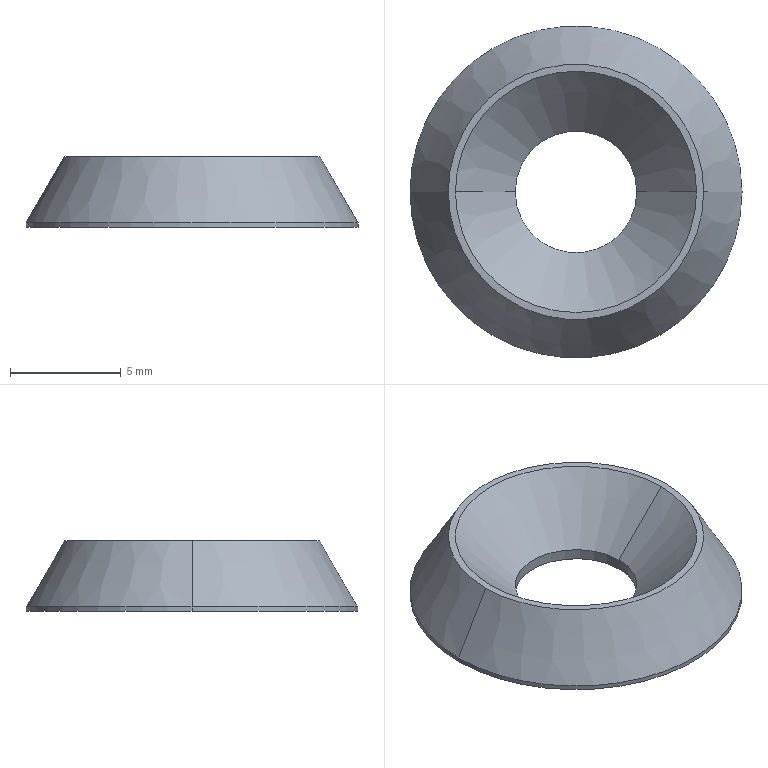Part | STEP file | 1 solid | 10 faces | box 15 x 15 x 3.2 mm | volume 292.86 mm3 | cone 4 | cylinder 4 | plane 2 | commonest cylinder face diameters 5.5 x2 15 x2
STEP:
#1=CARTESIAN_POINT('',(0.,0.,0.));
#2=DIRECTION('',(0.,0.,1.));
#3=DIRECTION('',(1.,0.,0.));
#4=AXIS2_PLACEMENT_3D('',#1,#2,#3);
#5=CARTESIAN_POINT('',(5.768,0.,1.6));
#6=VERTEX_POINT('',#5);
#7=CARTESIAN_POINT('',(-5.768,0.,1.6));
#8=VERTEX_POINT('',#7);
#9=CARTESIAN_POINT('',(0.,0.,1.6));
#10=DIRECTION('',(0.,0.,1.));
#11=DIRECTION('',(1.,0.,0.));
#12=AXIS2_PLACEMENT_3D('',#9,#10,#11);
#13=CIRCLE('',#12,5.768);
#14=CARTESIAN_POINT('',(0.,0.,1.6));
#15=DIRECTION('',(0.,0.,-1.));
#16=DIRECTION('',(-1.,0.,0.));
#17=AXIS2_PLACEMENT_3D('',#14,#15,#16);
#18=CONICAL_SURFACE('',#17,5.768,0.5236);
#19=CARTESIAN_POINT('',(3.142,0.));
#20=DIRECTION('',(-1.,0.));
#21=VECTOR('',#20,1.);
#22=LINE('',#19,#21);
#23=(GEOMETRIC_REPRESENTATION_CONTEXT(2)PARAMETRIC_REPRESENTATION_CONTEXT()REPRESENTATION_CONTEXT('',''));
#24=DEFINITIONAL_REPRESENTATION('',(#22),#23);
#25=PCURVE('',#18,#24);
#26=CARTESIAN_POINT('',(0.,0.,1.6));
#27=DIRECTION('',(0.,0.,1.));
#28=DIRECTION('',(1.,0.,0.));
#29=AXIS2_PLACEMENT_3D('',#26,#27,#28);
#30=PLANE('',#29);
#31=CARTESIAN_POINT('',(0.,0.));
#32=DIRECTION('',(1.,0.));
#33=AXIS2_PLACEMENT_2D('',#31,#32);
#34=CIRCLE('',#33,5.768);
#35=(GEOMETRIC_REPRESENTATION_CONTEXT(2)PARAMETRIC_REPRESENTATION_CONTEXT()REPRESENTATION_CONTEXT('',''));
#36=DEFINITIONAL_REPRESENTATION('',(#34),#35);
#37=PCURVE('',#30,#36);
#38=SURFACE_CURVE('',#13,(#25,#37),.PCURVE_S1.);
#39=EDGE_CURVE('',#6,#8,#38,.T.);
#40=ORIENTED_EDGE('',*,*,#39,.F.);
#41=CARTESIAN_POINT('',(7.5,0.,-1.4));
#42=VERTEX_POINT('',#41);
#43=CARTESIAN_POINT('',(5.768,0.,1.6));
#44=DIRECTION('',(0.5,0.,-0.866));
#45=VECTOR('',#44,1.);
#46=LINE('',#43,#45);
#47=CARTESIAN_POINT('',(3.142,0.));
#48=DIRECTION('',(0.,1.));
#49=VECTOR('',#48,1.);
#50=LINE('',#47,#49);
#51=(GEOMETRIC_REPRESENTATION_CONTEXT(2)PARAMETRIC_REPRESENTATION_CONTEXT()REPRESENTATION_CONTEXT('',''));
#52=DEFINITIONAL_REPRESENTATION('',(#50),#51);
#53=PCURVE('',#18,#52);
#54=CARTESIAN_POINT('',(0.,0.,1.6));
#55=DIRECTION('',(0.,0.,-1.));
#56=DIRECTION('',(-1.,0.,0.));
#57=AXIS2_PLACEMENT_3D('',#54,#55,#56);
#58=CONICAL_SURFACE('',#57,5.768,0.5236);
#59=CARTESIAN_POINT('',(3.142,0.));
#60=DIRECTION('',(0.,1.));
#61=VECTOR('',#60,1.);
#62=LINE('',#59,#61);
#63=(GEOMETRIC_REPRESENTATION_CONTEXT(2)PARAMETRIC_REPRESENTATION_CONTEXT()REPRESENTATION_CONTEXT('',''));
#64=DEFINITIONAL_REPRESENTATION('',(#62),#63);
#65=PCURVE('',#58,#64);
#66=SURFACE_CURVE('',#46,(#53,#65),.PCURVE_S1.);
#67=EDGE_CURVE('',#6,#42,#66,.T.);
#68=ORIENTED_EDGE('',*,*,#67,.T.);
#69=CARTESIAN_POINT('',(-7.5,0.,-1.4));
#70=VERTEX_POINT('',#69);
#71=CARTESIAN_POINT('',(0.,0.,-1.4));
#72=DIRECTION('',(0.,0.,-1.));
#73=DIRECTION('',(1.,0.,0.));
#74=AXIS2_PLACEMENT_3D('',#71,#72,#73);
#75=CIRCLE('',#74,7.5);
#76=CARTESIAN_POINT('',(-3.142,3.));
#77=DIRECTION('',(1.,0.));
#78=VECTOR('',#77,1.);
#79=LINE('',#76,#78);
#80=(GEOMETRIC_REPRESENTATION_CONTEXT(2)PARAMETRIC_REPRESENTATION_CONTEXT()REPRESENTATION_CONTEXT('',''));
#81=DEFINITIONAL_REPRESENTATION('',(#79),#80);
#82=PCURVE('',#18,#81);
#83=CARTESIAN_POINT('',(0.,0.,1.6));
#84=DIRECTION('',(0.,0.,-1.));
#85=DIRECTION('',(-1.,0.,0.));
#86=AXIS2_PLACEMENT_3D('',#83,#84,#85);
#87=CYLINDRICAL_SURFACE('',#86,7.5);
#88=CARTESIAN_POINT('',(-3.142,3.));
#89=DIRECTION('',(1.,0.));
#90=VECTOR('',#89,1.);
#91=LINE('',#88,#90);
#92=(GEOMETRIC_REPRESENTATION_CONTEXT(2)PARAMETRIC_REPRESENTATION_CONTEXT()REPRESENTATION_CONTEXT('',''));
#93=DEFINITIONAL_REPRESENTATION('',(#91),#92);
#94=PCURVE('',#87,#93);
#95=SURFACE_CURVE('',#75,(#82,#94),.PCURVE_S1.);
#96=EDGE_CURVE('',#70,#42,#95,.T.);
#97=ORIENTED_EDGE('',*,*,#96,.F.);
#98=CARTESIAN_POINT('',(-5.768,0.,1.6));
#99=DIRECTION('',(-0.5,0.,-0.866));
#100=VECTOR('',#99,1.);
#101=LINE('',#98,#100);
#102=CARTESIAN_POINT('',(0.,0.));
#103=DIRECTION('',(0.,1.));
#104=VECTOR('',#103,1.);
#105=LINE('',#102,#104);
#106=(GEOMETRIC_REPRESENTATION_CONTEXT(2)PARAMETRIC_REPRESENTATION_CONTEXT()REPRESENTATION_CONTEXT('',''));
#107=DEFINITIONAL_REPRESENTATION('',(#105),#106);
#108=PCURVE('',#18,#107);
#109=CARTESIAN_POINT('',(6.283,0.));
#110=DIRECTION('',(0.,1.));
#111=VECTOR('',#110,1.);
#112=LINE('',#109,#111);
#113=(GEOMETRIC_REPRESENTATION_CONTEXT(2)PARAMETRIC_REPRESENTATION_CONTEXT()REPRESENTATION_CONTEXT('',''));
#114=DEFINITIONAL_REPRESENTATION('',(#112),#113);
#115=PCURVE('',#58,#114);
#116=SURFACE_CURVE('',#101,(#108,#115),.PCURVE_S1.);
#117=EDGE_CURVE('',#8,#70,#116,.T.);
#118=ORIENTED_EDGE('',*,*,#117,.F.);
#119=EDGE_LOOP('',(#40,#68,#97,#118));
#120=FACE_BOUND('',#119,.T.);
#121=ADVANCED_FACE('',(#120),#18,.T.);
#122=CARTESIAN_POINT('',(2.75,0.,-1.1));
#123=VERTEX_POINT('',#122);
#124=CARTESIAN_POINT('',(5.45,0.,1.6));
#125=VERTEX_POINT('',#124);
#126=CARTESIAN_POINT('',(2.75,0.,-1.1));
#127=DIRECTION('',(0.7071,0.,0.7071));
#128=VECTOR('',#127,1.);
#129=LINE('',#126,#128);
#130=CARTESIAN_POINT('',(0.,0.,-1.1));
#131=DIRECTION('',(0.,0.,1.));
#132=DIRECTION('',(1.,0.,0.));
#133=AXIS2_PLACEMENT_3D('',#130,#131,#132);
#134=CONICAL_SURFACE('',#133,2.75,0.7854);
#135=CARTESIAN_POINT('',(6.283,0.));
#136=DIRECTION('',(0.,1.));
#137=VECTOR('',#136,1.);
#138=LINE('',#135,#137);
#139=(GEOMETRIC_REPRESENTATION_CONTEXT(2)PARAMETRIC_REPRESENTATION_CONTEXT()REPRESENTATION_CONTEXT('',''));
#140=DEFINITIONAL_REPRESENTATION('',(#138),#139);
#141=PCURVE('',#134,#140);
#142=CARTESIAN_POINT('',(0.,0.,-1.1));
#143=DIRECTION('',(0.,0.,1.));
#144=DIRECTION('',(1.,0.,0.));
#145=AXIS2_PLACEMENT_3D('',#142,#143,#144);
#146=CONICAL_SURFACE('',#145,2.75,0.7854);
#147=CARTESIAN_POINT('',(0.,0.));
#148=DIRECTION('',(0.,1.));
#149=VECTOR('',#148,1.);
#150=LINE('',#147,#149);
#151=(GEOMETRIC_REPRESENTATION_CONTEXT(2)PARAMETRIC_REPRESENTATION_CONTEXT()REPRESENTATION_CONTEXT('',''));
#152=DEFINITIONAL_REPRESENTATION('',(#150),#151);
#153=PCURVE('',#146,#152);
#154=SURFACE_CURVE('',#129,(#141,#153),.PCURVE_S1.);
#155=EDGE_CURVE('',#123,#125,#154,.T.);
#156=ORIENTED_EDGE('',*,*,#155,.T.);
#157=CARTESIAN_POINT('',(-5.45,0.,1.6));
#158=VERTEX_POINT('',#157);
#159=CARTESIAN_POINT('',(0.,0.,1.6));
#160=DIRECTION('',(0.,0.,-1.));
#161=DIRECTION('',(1.,0.,0.));
#162=AXIS2_PLACEMENT_3D('',#159,#160,#161);
#163=CIRCLE('',#162,5.45);
#164=CARTESIAN_POINT('',(6.283,2.7));
#165=DIRECTION('',(-1.,0.));
#166=VECTOR('',#165,1.);
#167=LINE('',#164,#166);
#168=(GEOMETRIC_REPRESENTATION_CONTEXT(2)PARAMETRIC_REPRESENTATION_CONTEXT()REPRESENTATION_CONTEXT('',''));
#169=DEFINITIONAL_REPRESENTATION('',(#167),#168);
#170=PCURVE('',#134,#169);
#171=CARTESIAN_POINT('',(5.45,0.));
#172=CARTESIAN_POINT('',(5.45,-9.44));
#173=CARTESIAN_POINT('',(-2.725,-4.72));
#174=CARTESIAN_POINT('',(-10.9,0.));
#175=CARTESIAN_POINT('',(-2.725,4.72));
#176=CARTESIAN_POINT('',(5.45,9.44));
#177=CARTESIAN_POINT('',(5.45,0.));
#178=(BOUNDED_CURVE()B_SPLINE_CURVE(2,(#171,#172,#173,#174,#175,#176,#177),.UNSPECIFIED.,.T.,.F.)B_SPLINE_CURVE_WITH_KNOTS((1,2,2,2,2,1),(-2.094,0.,2.094,4.189,6.283,8.378),.UNSPECIFIED.)CURVE()GEOMETRIC_REPRESENTATION_ITEM()RATIONAL_B_SPLINE_CURVE((1.,0.5,1.,0.5,1.,0.5,1.))REPRESENTATION_ITEM(''));
#179=(GEOMETRIC_REPRESENTATION_CONTEXT(2)PARAMETRIC_REPRESENTATION_CONTEXT()REPRESENTATION_CONTEXT('',''));
#180=DEFINITIONAL_REPRESENTATION('',(#178),#179);
#181=PCURVE('',#30,#180);
#182=SURFACE_CURVE('',#163,(#170,#181),.PCURVE_S1.);
#183=EDGE_CURVE('',#125,#158,#182,.T.);
#184=ORIENTED_EDGE('',*,*,#183,.T.);
#185=CARTESIAN_POINT('',(-2.75,0.,-1.1));
#186=VERTEX_POINT('',#185);
#187=CARTESIAN_POINT('',(-2.75,0.,-1.1));
#188=DIRECTION('',(-0.7071,0.,0.7071));
#189=VECTOR('',#188,1.);
#190=LINE('',#187,#189);
#191=CARTESIAN_POINT('',(3.142,0.));
#192=DIRECTION('',(0.,1.));
#193=VECTOR('',#192,1.);
#194=LINE('',#191,#193);
#195=(GEOMETRIC_REPRESENTATION_CONTEXT(2)PARAMETRIC_REPRESENTATION_CONTEXT()REPRESENTATION_CONTEXT('',''));
#196=DEFINITIONAL_REPRESENTATION('',(#194),#195);
#197=PCURVE('',#134,#196);
#198=CARTESIAN_POINT('',(3.142,0.));
#199=DIRECTION('',(0.,1.));
#200=VECTOR('',#199,1.);
#201=LINE('',#198,#200);
#202=(GEOMETRIC_REPRESENTATION_CONTEXT(2)PARAMETRIC_REPRESENTATION_CONTEXT()REPRESENTATION_CONTEXT('',''));
#203=DEFINITIONAL_REPRESENTATION('',(#201),#202);
#204=PCURVE('',#146,#203);
#205=SURFACE_CURVE('',#190,(#197,#204),.PCURVE_S1.);
#206=EDGE_CURVE('',#186,#158,#205,.T.);
#207=ORIENTED_EDGE('',*,*,#206,.F.);
#208=CARTESIAN_POINT('',(0.,0.,-1.1));
#209=DIRECTION('',(0.,0.,1.));
#210=DIRECTION('',(1.,0.,0.));
#211=AXIS2_PLACEMENT_3D('',#208,#209,#210);
#212=CIRCLE('',#211,2.75);
#213=CARTESIAN_POINT('',(0.,0.));
#214=DIRECTION('',(1.,0.));
#215=VECTOR('',#214,1.);
#216=LINE('',#213,#215);
#217=(GEOMETRIC_REPRESENTATION_CONTEXT(2)PARAMETRIC_REPRESENTATION_CONTEXT()REPRESENTATION_CONTEXT('',''));
#218=DEFINITIONAL_REPRESENTATION('',(#216),#217);
#219=PCURVE('',#134,#218);
#220=CARTESIAN_POINT('',(0.,0.,1.6));
#221=DIRECTION('',(0.,0.,-1.));
#222=DIRECTION('',(-1.,0.,0.));
#223=AXIS2_PLACEMENT_3D('',#220,#221,#222);
#224=CYLINDRICAL_SURFACE('',#223,2.75);
#225=CARTESIAN_POINT('',(9.425,2.7));
#226=DIRECTION('',(-1.,0.));
#227=VECTOR('',#226,1.);
#228=LINE('',#225,#227);
#229=(GEOMETRIC_REPRESENTATION_CONTEXT(2)PARAMETRIC_REPRESENTATION_CONTEXT()REPRESENTATION_CONTEXT('',''));
#230=DEFINITIONAL_REPRESENTATION('',(#228),#229);
#231=PCURVE('',#224,#230);
#232=SURFACE_CURVE('',#212,(#219,#231),.PCURVE_S1.);
#233=EDGE_CURVE('',#186,#123,#232,.T.);
#234=ORIENTED_EDGE('',*,*,#233,.T.);
#235=EDGE_LOOP('',(#156,#184,#207,#234));
#236=FACE_BOUND('',#235,.F.);
#237=ADVANCED_FACE('',(#236),#134,.F.);
#238=CARTESIAN_POINT('',(-2.75,0.,-1.6));
#239=VERTEX_POINT('',#238);
#240=CARTESIAN_POINT('',(-2.75,0.,1.6));
#241=DIRECTION('',(0.,0.,-1.));
#242=VECTOR('',#241,1.);
#243=LINE('',#240,#242);
#244=CARTESIAN_POINT('',(6.283,0.));
#245=DIRECTION('',(0.,1.));
#246=VECTOR('',#245,1.);
#247=LINE('',#244,#246);
#248=(GEOMETRIC_REPRESENTATION_CONTEXT(2)PARAMETRIC_REPRESENTATION_CONTEXT()REPRESENTATION_CONTEXT('',''));
#249=DEFINITIONAL_REPRESENTATION('',(#247),#248);
#250=PCURVE('',#224,#249);
#251=CARTESIAN_POINT('',(0.,0.,1.6));
#252=DIRECTION('',(0.,0.,-1.));
#253=DIRECTION('',(-1.,0.,0.));
#254=AXIS2_PLACEMENT_3D('',#251,#252,#253);
#255=CYLINDRICAL_SURFACE('',#254,2.75);
#256=CARTESIAN_POINT('',(0.,0.));
#257=DIRECTION('',(0.,1.));
#258=VECTOR('',#257,1.);
#259=LINE('',#256,#258);
#260=(GEOMETRIC_REPRESENTATION_CONTEXT(2)PARAMETRIC_REPRESENTATION_CONTEXT()REPRESENTATION_CONTEXT('',''));
#261=DEFINITIONAL_REPRESENTATION('',(#259),#260);
#262=PCURVE('',#255,#261);
#263=SURFACE_CURVE('',#243,(#250,#262),.PCURVE_S1.);
#264=EDGE_CURVE('',#186,#239,#263,.T.);
#265=ORIENTED_EDGE('',*,*,#264,.T.);
#266=CARTESIAN_POINT('',(2.75,0.,-1.6));
#267=VERTEX_POINT('',#266);
#268=CARTESIAN_POINT('',(0.,0.,-1.6));
#269=DIRECTION('',(0.,0.,1.));
#270=DIRECTION('',(1.,0.,0.));
#271=AXIS2_PLACEMENT_3D('',#268,#269,#270);
#272=CIRCLE('',#271,2.75);
#273=CARTESIAN_POINT('',(9.425,3.2));
#274=DIRECTION('',(-1.,0.));
#275=VECTOR('',#274,1.);
#276=LINE('',#273,#275);
#277=(GEOMETRIC_REPRESENTATION_CONTEXT(2)PARAMETRIC_REPRESENTATION_CONTEXT()REPRESENTATION_CONTEXT('',''));
#278=DEFINITIONAL_REPRESENTATION('',(#276),#277);
#279=PCURVE('',#224,#278);
#280=CARTESIAN_POINT('',(0.,0.,-1.6));
#281=DIRECTION('',(0.,0.,1.));
#282=DIRECTION('',(1.,0.,0.));
#283=AXIS2_PLACEMENT_3D('',#280,#281,#282);
#284=PLANE('',#283);
#285=CARTESIAN_POINT('',(0.,0.));
#286=DIRECTION('',(1.,0.));
#287=AXIS2_PLACEMENT_2D('',#285,#286);
#288=CIRCLE('',#287,2.75);
#289=(GEOMETRIC_REPRESENTATION_CONTEXT(2)PARAMETRIC_REPRESENTATION_CONTEXT()REPRESENTATION_CONTEXT('',''));
#290=DEFINITIONAL_REPRESENTATION('',(#288),#289);
#291=PCURVE('',#284,#290);
#292=SURFACE_CURVE('',#272,(#279,#291),.PCURVE_S1.);
#293=EDGE_CURVE('',#239,#267,#292,.T.);
#294=ORIENTED_EDGE('',*,*,#293,.T.);
#295=CARTESIAN_POINT('',(2.75,0.,1.6));
#296=DIRECTION('',(0.,0.,-1.));
#297=VECTOR('',#296,1.);
#298=LINE('',#295,#297);
#299=CARTESIAN_POINT('',(3.142,0.));
#300=DIRECTION('',(0.,1.));
#301=VECTOR('',#300,1.);
#302=LINE('',#299,#301);
#303=(GEOMETRIC_REPRESENTATION_CONTEXT(2)PARAMETRIC_REPRESENTATION_CONTEXT()REPRESENTATION_CONTEXT('',''));
#304=DEFINITIONAL_REPRESENTATION('',(#302),#303);
#305=PCURVE('',#224,#304);
#306=CARTESIAN_POINT('',(3.142,0.));
#307=DIRECTION('',(0.,1.));
#308=VECTOR('',#307,1.);
#309=LINE('',#306,#308);
#310=(GEOMETRIC_REPRESENTATION_CONTEXT(2)PARAMETRIC_REPRESENTATION_CONTEXT()REPRESENTATION_CONTEXT('',''));
#311=DEFINITIONAL_REPRESENTATION('',(#309),#310);
#312=PCURVE('',#255,#311);
#313=SURFACE_CURVE('',#298,(#305,#312),.PCURVE_S1.);
#314=EDGE_CURVE('',#123,#267,#313,.T.);
#315=ORIENTED_EDGE('',*,*,#314,.F.);
#316=ORIENTED_EDGE('',*,*,#233,.F.);
#317=EDGE_LOOP('',(#265,#294,#315,#316));
#318=FACE_BOUND('',#317,.F.);
#319=ADVANCED_FACE('',(#318),#224,.F.);
#320=ORIENTED_EDGE('',*,*,#96,.T.);
#321=CARTESIAN_POINT('',(7.5,0.,-1.6));
#322=VERTEX_POINT('',#321);
#323=CARTESIAN_POINT('',(7.5,0.,1.6));
#324=DIRECTION('',(0.,0.,-1.));
#325=VECTOR('',#324,1.);
#326=LINE('',#323,#325);
#327=CARTESIAN_POINT('',(3.142,0.));
#328=DIRECTION('',(0.,1.));
#329=VECTOR('',#328,1.);
#330=LINE('',#327,#329);
#331=(GEOMETRIC_REPRESENTATION_CONTEXT(2)PARAMETRIC_REPRESENTATION_CONTEXT()REPRESENTATION_CONTEXT('',''));
#332=DEFINITIONAL_REPRESENTATION('',(#330),#331);
#333=PCURVE('',#87,#332);
#334=CARTESIAN_POINT('',(0.,0.,1.6));
#335=DIRECTION('',(0.,0.,-1.));
#336=DIRECTION('',(-1.,0.,0.));
#337=AXIS2_PLACEMENT_3D('',#334,#335,#336);
#338=CYLINDRICAL_SURFACE('',#337,7.5);
#339=CARTESIAN_POINT('',(3.142,0.));
#340=DIRECTION('',(0.,1.));
#341=VECTOR('',#340,1.);
#342=LINE('',#339,#341);
#343=(GEOMETRIC_REPRESENTATION_CONTEXT(2)PARAMETRIC_REPRESENTATION_CONTEXT()REPRESENTATION_CONTEXT('',''));
#344=DEFINITIONAL_REPRESENTATION('',(#342),#343);
#345=PCURVE('',#338,#344);
#346=SURFACE_CURVE('',#326,(#333,#345),.PCURVE_S1.);
#347=EDGE_CURVE('',#42,#322,#346,.T.);
#348=ORIENTED_EDGE('',*,*,#347,.T.);
#349=CARTESIAN_POINT('',(-7.5,0.,-1.6));
#350=VERTEX_POINT('',#349);
#351=CARTESIAN_POINT('',(0.,0.,-1.6));
#352=DIRECTION('',(0.,0.,1.));
#353=DIRECTION('',(1.,0.,0.));
#354=AXIS2_PLACEMENT_3D('',#351,#352,#353);
#355=CIRCLE('',#354,7.5);
#356=CARTESIAN_POINT('',(3.142,3.2));
#357=DIRECTION('',(-1.,0.));
#358=VECTOR('',#357,1.);
#359=LINE('',#356,#358);
#360=(GEOMETRIC_REPRESENTATION_CONTEXT(2)PARAMETRIC_REPRESENTATION_CONTEXT()REPRESENTATION_CONTEXT('',''));
#361=DEFINITIONAL_REPRESENTATION('',(#359),#360);
#362=PCURVE('',#87,#361);
#363=CARTESIAN_POINT('',(0.,0.));
#364=DIRECTION('',(1.,0.));
#365=AXIS2_PLACEMENT_2D('',#363,#364);
#366=CIRCLE('',#365,7.5);
#367=(GEOMETRIC_REPRESENTATION_CONTEXT(2)PARAMETRIC_REPRESENTATION_CONTEXT()REPRESENTATION_CONTEXT('',''));
#368=DEFINITIONAL_REPRESENTATION('',(#366),#367);
#369=PCURVE('',#284,#368);
#370=SURFACE_CURVE('',#355,(#362,#369),.PCURVE_S1.);
#371=EDGE_CURVE('',#322,#350,#370,.T.);
#372=ORIENTED_EDGE('',*,*,#371,.T.);
#373=CARTESIAN_POINT('',(-7.5,0.,1.6));
#374=DIRECTION('',(0.,0.,-1.));
#375=VECTOR('',#374,1.);
#376=LINE('',#373,#375);
#377=CARTESIAN_POINT('',(0.,0.));
#378=DIRECTION('',(0.,1.));
#379=VECTOR('',#378,1.);
#380=LINE('',#377,#379);
#381=(GEOMETRIC_REPRESENTATION_CONTEXT(2)PARAMETRIC_REPRESENTATION_CONTEXT()REPRESENTATION_CONTEXT('',''));
#382=DEFINITIONAL_REPRESENTATION('',(#380),#381);
#383=PCURVE('',#87,#382);
#384=CARTESIAN_POINT('',(6.283,0.));
#385=DIRECTION('',(0.,1.));
#386=VECTOR('',#385,1.);
#387=LINE('',#384,#386);
#388=(GEOMETRIC_REPRESENTATION_CONTEXT(2)PARAMETRIC_REPRESENTATION_CONTEXT()REPRESENTATION_CONTEXT('',''));
#389=DEFINITIONAL_REPRESENTATION('',(#387),#388);
#390=PCURVE('',#338,#389);
#391=SURFACE_CURVE('',#376,(#383,#390),.PCURVE_S1.);
#392=EDGE_CURVE('',#70,#350,#391,.T.);
#393=ORIENTED_EDGE('',*,*,#392,.F.);
#394=EDGE_LOOP('',(#320,#348,#372,#393));
#395=FACE_BOUND('',#394,.T.);
#396=ADVANCED_FACE('',(#395),#87,.T.);
#397=CARTESIAN_POINT('',(0.,0.,1.6));
#398=DIRECTION('',(0.,0.,1.));
#399=DIRECTION('',(1.,0.,0.));
#400=AXIS2_PLACEMENT_3D('',#397,#398,#399);
#401=CIRCLE('',#400,5.768);
#402=CARTESIAN_POINT('',(0.,0.));
#403=DIRECTION('',(1.,0.));
#404=AXIS2_PLACEMENT_2D('',#402,#403);
#405=CIRCLE('',#404,5.768);
#406=(GEOMETRIC_REPRESENTATION_CONTEXT(2)PARAMETRIC_REPRESENTATION_CONTEXT()REPRESENTATION_CONTEXT('',''));
#407=DEFINITIONAL_REPRESENTATION('',(#405),#406);
#408=PCURVE('',#30,#407);
#409=CARTESIAN_POINT('',(9.425,0.));
#410=DIRECTION('',(-1.,0.));
#411=VECTOR('',#410,1.);
#412=LINE('',#409,#411);
#413=(GEOMETRIC_REPRESENTATION_CONTEXT(2)PARAMETRIC_REPRESENTATION_CONTEXT()REPRESENTATION_CONTEXT('',''));
#414=DEFINITIONAL_REPRESENTATION('',(#412),#413);
#415=PCURVE('',#58,#414);
#416=SURFACE_CURVE('',#401,(#408,#415),.PCURVE_S1.);
#417=EDGE_CURVE('',#8,#6,#416,.T.);
#418=ORIENTED_EDGE('',*,*,#417,.T.);
#419=ORIENTED_EDGE('',*,*,#39,.T.);
#420=EDGE_LOOP('',(#418,#419));
#421=FACE_BOUND('',#420,.T.);
#422=ORIENTED_EDGE('',*,*,#183,.T.);
#423=CARTESIAN_POINT('',(0.,0.,1.6));
#424=DIRECTION('',(0.,0.,-1.));
#425=DIRECTION('',(1.,0.,0.));
#426=AXIS2_PLACEMENT_3D('',#423,#424,#425);
#427=CIRCLE('',#426,5.45);
#428=CARTESIAN_POINT('',(5.45,0.));
#429=CARTESIAN_POINT('',(5.45,-9.44));
#430=CARTESIAN_POINT('',(-2.725,-4.72));
#431=CARTESIAN_POINT('',(-10.9,0.));
#432=CARTESIAN_POINT('',(-2.725,4.72));
#433=CARTESIAN_POINT('',(5.45,9.44));
#434=CARTESIAN_POINT('',(5.45,0.));
#435=(BOUNDED_CURVE()B_SPLINE_CURVE(2,(#428,#429,#430,#431,#432,#433,#434),.UNSPECIFIED.,.T.,.F.)B_SPLINE_CURVE_WITH_KNOTS((1,2,2,2,2,1),(-2.094,0.,2.094,4.189,6.283,8.378),.UNSPECIFIED.)CURVE()GEOMETRIC_REPRESENTATION_ITEM()RATIONAL_B_SPLINE_CURVE((1.,0.5,1.,0.5,1.,0.5,1.))REPRESENTATION_ITEM(''));
#436=(GEOMETRIC_REPRESENTATION_CONTEXT(2)PARAMETRIC_REPRESENTATION_CONTEXT()REPRESENTATION_CONTEXT('',''));
#437=DEFINITIONAL_REPRESENTATION('',(#435),#436);
#438=PCURVE('',#30,#437);
#439=CARTESIAN_POINT('',(6.283,2.7));
#440=DIRECTION('',(-1.,0.));
#441=VECTOR('',#440,1.);
#442=LINE('',#439,#441);
#443=(GEOMETRIC_REPRESENTATION_CONTEXT(2)PARAMETRIC_REPRESENTATION_CONTEXT()REPRESENTATION_CONTEXT('',''));
#444=DEFINITIONAL_REPRESENTATION('',(#442),#443);
#445=PCURVE('',#146,#444);
#446=SURFACE_CURVE('',#427,(#438,#445),.PCURVE_S1.);
#447=EDGE_CURVE('',#158,#125,#446,.T.);
#448=ORIENTED_EDGE('',*,*,#447,.T.);
#449=EDGE_LOOP('',(#422,#448));
#450=FACE_BOUND('',#449,.T.);
#451=ADVANCED_FACE('',(#421,#450),#30,.T.);
#452=CARTESIAN_POINT('',(0.,0.,-1.6));
#453=DIRECTION('',(0.,0.,1.));
#454=DIRECTION('',(1.,0.,0.));
#455=AXIS2_PLACEMENT_3D('',#452,#453,#454);
#456=CIRCLE('',#455,7.5);
#457=CARTESIAN_POINT('',(0.,0.));
#458=DIRECTION('',(1.,0.));
#459=AXIS2_PLACEMENT_2D('',#457,#458);
#460=CIRCLE('',#459,7.5);
#461=(GEOMETRIC_REPRESENTATION_CONTEXT(2)PARAMETRIC_REPRESENTATION_CONTEXT()REPRESENTATION_CONTEXT('',''));
#462=DEFINITIONAL_REPRESENTATION('',(#460),#461);
#463=PCURVE('',#284,#462);
#464=CARTESIAN_POINT('',(9.425,3.2));
#465=DIRECTION('',(-1.,0.));
#466=VECTOR('',#465,1.);
#467=LINE('',#464,#466);
#468=(GEOMETRIC_REPRESENTATION_CONTEXT(2)PARAMETRIC_REPRESENTATION_CONTEXT()REPRESENTATION_CONTEXT('',''));
#469=DEFINITIONAL_REPRESENTATION('',(#467),#468);
#470=PCURVE('',#338,#469);
#471=SURFACE_CURVE('',#456,(#463,#470),.PCURVE_S1.);
#472=EDGE_CURVE('',#350,#322,#471,.T.);
#473=ORIENTED_EDGE('',*,*,#472,.F.);
#474=ORIENTED_EDGE('',*,*,#371,.F.);
#475=EDGE_LOOP('',(#473,#474));
#476=FACE_BOUND('',#475,.T.);
#477=ORIENTED_EDGE('',*,*,#293,.T.);
#478=CARTESIAN_POINT('',(0.,0.,-1.6));
#479=DIRECTION('',(0.,0.,1.));
#480=DIRECTION('',(1.,0.,0.));
#481=AXIS2_PLACEMENT_3D('',#478,#479,#480);
#482=CIRCLE('',#481,2.75);
#483=CARTESIAN_POINT('',(0.,0.));
#484=DIRECTION('',(1.,0.));
#485=AXIS2_PLACEMENT_2D('',#483,#484);
#486=CIRCLE('',#485,2.75);
#487=(GEOMETRIC_REPRESENTATION_CONTEXT(2)PARAMETRIC_REPRESENTATION_CONTEXT()REPRESENTATION_CONTEXT('',''));
#488=DEFINITIONAL_REPRESENTATION('',(#486),#487);
#489=PCURVE('',#284,#488);
#490=CARTESIAN_POINT('',(3.142,3.2));
#491=DIRECTION('',(-1.,0.));
#492=VECTOR('',#491,1.);
#493=LINE('',#490,#492);
#494=(GEOMETRIC_REPRESENTATION_CONTEXT(2)PARAMETRIC_REPRESENTATION_CONTEXT()REPRESENTATION_CONTEXT('',''));
#495=DEFINITIONAL_REPRESENTATION('',(#493),#494);
#496=PCURVE('',#255,#495);
#497=SURFACE_CURVE('',#482,(#489,#496),.PCURVE_S1.);
#498=EDGE_CURVE('',#267,#239,#497,.T.);
#499=ORIENTED_EDGE('',*,*,#498,.T.);
#500=EDGE_LOOP('',(#477,#499));
#501=FACE_BOUND('',#500,.T.);
#502=ADVANCED_FACE('',(#476,#501),#284,.F.);
#503=ORIENTED_EDGE('',*,*,#347,.F.);
#504=CARTESIAN_POINT('',(0.,0.,-1.4));
#505=DIRECTION('',(0.,0.,-1.));
#506=DIRECTION('',(1.,0.,0.));
#507=AXIS2_PLACEMENT_3D('',#504,#505,#506);
#508=CIRCLE('',#507,7.5);
#509=CARTESIAN_POINT('',(3.142,3.));
#510=DIRECTION('',(1.,0.));
#511=VECTOR('',#510,1.);
#512=LINE('',#509,#511);
#513=(GEOMETRIC_REPRESENTATION_CONTEXT(2)PARAMETRIC_REPRESENTATION_CONTEXT()REPRESENTATION_CONTEXT('',''));
#514=DEFINITIONAL_REPRESENTATION('',(#512),#513);
#515=PCURVE('',#338,#514);
#516=CARTESIAN_POINT('',(3.142,3.));
#517=DIRECTION('',(1.,0.));
#518=VECTOR('',#517,1.);
#519=LINE('',#516,#518);
#520=(GEOMETRIC_REPRESENTATION_CONTEXT(2)PARAMETRIC_REPRESENTATION_CONTEXT()REPRESENTATION_CONTEXT('',''));
#521=DEFINITIONAL_REPRESENTATION('',(#519),#520);
#522=PCURVE('',#58,#521);
#523=SURFACE_CURVE('',#508,(#515,#522),.PCURVE_S1.);
#524=EDGE_CURVE('',#42,#70,#523,.T.);
#525=ORIENTED_EDGE('',*,*,#524,.T.);
#526=ORIENTED_EDGE('',*,*,#392,.T.);
#527=ORIENTED_EDGE('',*,*,#472,.T.);
#528=EDGE_LOOP('',(#503,#525,#526,#527));
#529=FACE_BOUND('',#528,.T.);
#530=ADVANCED_FACE('',(#529),#338,.T.);
#531=ORIENTED_EDGE('',*,*,#498,.T.);
#532=ORIENTED_EDGE('',*,*,#264,.F.);
#533=CARTESIAN_POINT('',(0.,0.,-1.1));
#534=DIRECTION('',(0.,0.,1.));
#535=DIRECTION('',(1.,0.,0.));
#536=AXIS2_PLACEMENT_3D('',#533,#534,#535);
#537=CIRCLE('',#536,2.75);
#538=CARTESIAN_POINT('',(3.142,2.7));
#539=DIRECTION('',(-1.,0.));
#540=VECTOR('',#539,1.);
#541=LINE('',#538,#540);
#542=(GEOMETRIC_REPRESENTATION_CONTEXT(2)PARAMETRIC_REPRESENTATION_CONTEXT()REPRESENTATION_CONTEXT('',''));
#543=DEFINITIONAL_REPRESENTATION('',(#541),#542);
#544=PCURVE('',#255,#543);
#545=CARTESIAN_POINT('',(0.,0.));
#546=DIRECTION('',(1.,0.));
#547=VECTOR('',#546,1.);
#548=LINE('',#545,#547);
#549=(GEOMETRIC_REPRESENTATION_CONTEXT(2)PARAMETRIC_REPRESENTATION_CONTEXT()REPRESENTATION_CONTEXT('',''));
#550=DEFINITIONAL_REPRESENTATION('',(#548),#549);
#551=PCURVE('',#146,#550);
#552=SURFACE_CURVE('',#537,(#544,#551),.PCURVE_S1.);
#553=EDGE_CURVE('',#123,#186,#552,.T.);
#554=ORIENTED_EDGE('',*,*,#553,.F.);
#555=ORIENTED_EDGE('',*,*,#314,.T.);
#556=EDGE_LOOP('',(#531,#532,#554,#555));
#557=FACE_BOUND('',#556,.F.);
#558=ADVANCED_FACE('',(#557),#255,.F.);
#559=ORIENTED_EDGE('',*,*,#447,.T.);
#560=ORIENTED_EDGE('',*,*,#155,.F.);
#561=ORIENTED_EDGE('',*,*,#553,.T.);
#562=ORIENTED_EDGE('',*,*,#206,.T.);
#563=EDGE_LOOP('',(#559,#560,#561,#562));
#564=FACE_BOUND('',#563,.F.);
#565=ADVANCED_FACE('',(#564),#146,.F.);
#566=ORIENTED_EDGE('',*,*,#67,.F.);
#567=ORIENTED_EDGE('',*,*,#417,.F.);
#568=ORIENTED_EDGE('',*,*,#117,.T.);
#569=ORIENTED_EDGE('',*,*,#524,.F.);
#570=EDGE_LOOP('',(#566,#567,#568,#569));
#571=FACE_BOUND('',#570,.T.);
#572=ADVANCED_FACE('',(#571),#58,.T.);
#573=CLOSED_SHELL('',(#121,#237,#319,#396,#451,#502,#530,#558,#565,#572));
#574=MANIFOLD_SOLID_BREP('',#573);
#575=(LENGTH_UNIT()NAMED_UNIT(*)SI_UNIT(.MILLI.,.METRE.));
#576=UNCERTAINTY_MEASURE_WITH_UNIT(LENGTH_MEASURE(0.0000001),#575,'','');
#577=(NAMED_UNIT(*)PLANE_ANGLE_UNIT()SI_UNIT($,.RADIAN.));
#578=(NAMED_UNIT(*)SI_UNIT($,.STERADIAN.)SOLID_ANGLE_UNIT());
#579=(GEOMETRIC_REPRESENTATION_CONTEXT(3)GLOBAL_UNCERTAINTY_ASSIGNED_CONTEXT((#576))GLOBAL_UNIT_ASSIGNED_CONTEXT((#575,#577,#578))REPRESENTATION_CONTEXT('',''));
#580=ADVANCED_BREP_SHAPE_REPRESENTATION('',(#4,#574),#579);